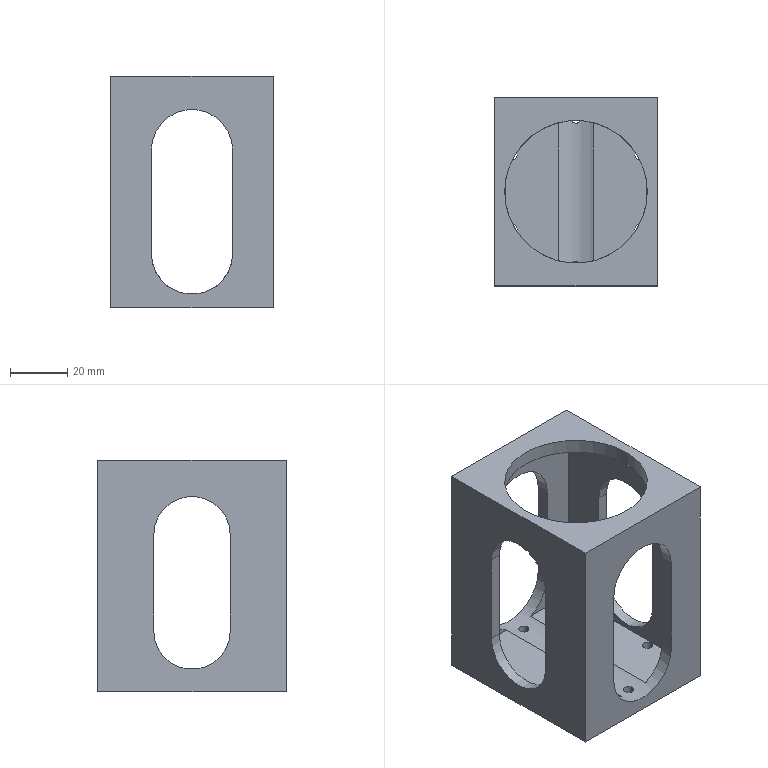Part | STEP file | 2026.6.15-Main Assembly图.sldasm-Part-160 | 1 solid | 45 faces | box 57 x 66 x 81 mm | volume 71126 mm3 | plane 24 | cylinder 21 | commonest cylinder face diameters 3.6 x12 26.76 x4 28.502 x3 50 x2